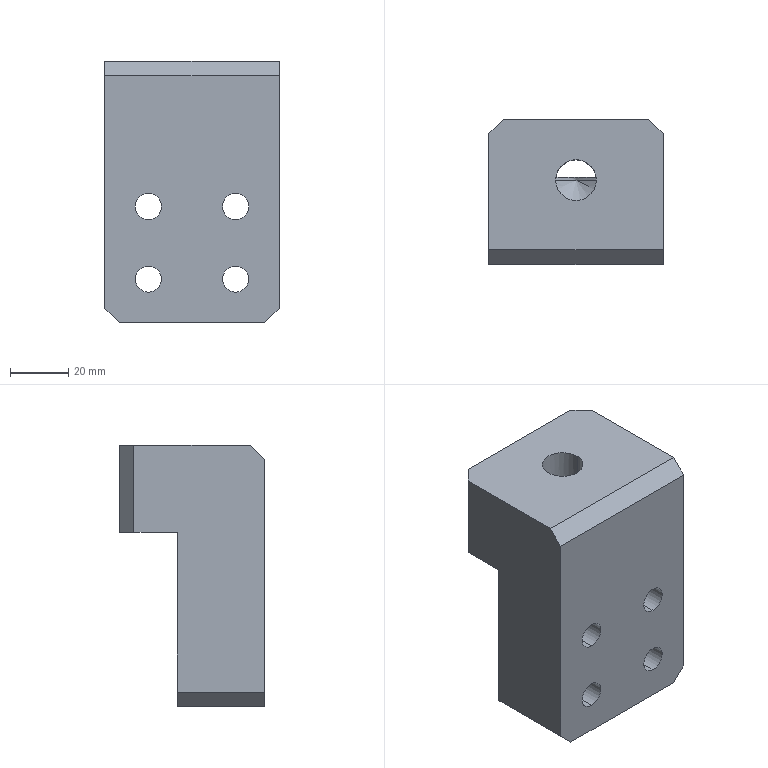Part | SolidWorks | features Chamfer 2, HoleWzd 2, Extrusion 1, ICE 1 | 1 solid | 25 faces | box 60 x 50 x 90 mm | volume 182634 mm3 | plane 13 | cylinder 10 | cone 2 | commonest cylinder face diameters 9 x8 14 x2
STEP:
#1=CARTESIAN_POINT('',(0.,14.,47.794));
#2=VERTEX_POINT('',#1);
#3=CARTESIAN_POINT('',(7.,14.,52.));
#4=VERTEX_POINT('',#3);
#5=CARTESIAN_POINT('',(7.,14.,52.));
#6=DIRECTION('',(0.8572,0.,0.515));
#7=VECTOR('',#6,1000.);
#8=LINE('',#5,#7);
#9=EDGE_CURVE('',#2,#4,#8,.T.);
#10=ORIENTED_EDGE('',*,*,#9,.F.);
#11=CARTESIAN_POINT('',(-7.,14.,52.));
#12=VERTEX_POINT('',#11);
#13=CARTESIAN_POINT('',(-7.,14.,52.));
#14=DIRECTION('',(-0.8572,0.,0.515));
#15=VECTOR('',#14,1000.);
#16=LINE('',#13,#15);
#17=EDGE_CURVE('',#2,#12,#16,.T.);
#18=ORIENTED_EDGE('',*,*,#17,.T.);
#19=CARTESIAN_POINT('',(0.,14.,52.));
#20=DIRECTION('',(0.,0.,1.));
#21=DIRECTION('',(1.,0.,0.));
#22=AXIS2_PLACEMENT_3D('',#19,#20,#21);
#23=CIRCLE('',#22,7.);
#24=EDGE_CURVE('',#12,#4,#23,.T.);
#25=ORIENTED_EDGE('',*,*,#24,.T.);
#26=EDGE_LOOP('',(#10,#18,#25));
#27=FACE_OUTER_BOUND('',#26,.T.);
#28=CARTESIAN_POINT('',(0.,14.,52.));
#29=DIRECTION('',(0.,0.,1.));
#30=DIRECTION('',(1.,0.,0.));
#31=AXIS2_PLACEMENT_3D('',#28,#29,#30);
#32=CONICAL_SURFACE('',#31,7.,1.03);
#33=ADVANCED_FACE('',(#27),#32,.F.);
#34=ORIENTED_EDGE('',*,*,#24,.F.);
#35=CARTESIAN_POINT('',(-7.,14.,90.));
#36=VERTEX_POINT('',#35);
#37=CARTESIAN_POINT('',(-7.,14.,90.));
#38=DIRECTION('',(0.,0.,1.));
#39=VECTOR('',#38,1000.);
#40=LINE('',#37,#39);
#41=EDGE_CURVE('',#12,#36,#40,.T.);
#42=ORIENTED_EDGE('',*,*,#41,.T.);
#43=CARTESIAN_POINT('',(7.,14.,90.));
#44=VERTEX_POINT('',#43);
#45=CARTESIAN_POINT('',(0.,14.,90.));
#46=DIRECTION('',(0.,0.,1.));
#47=DIRECTION('',(1.,0.,0.));
#48=AXIS2_PLACEMENT_3D('',#45,#46,#47);
#49=CIRCLE('',#48,7.);
#50=EDGE_CURVE('',#36,#44,#49,.T.);
#51=ORIENTED_EDGE('',*,*,#50,.T.);
#52=CARTESIAN_POINT('',(7.,14.,90.));
#53=DIRECTION('',(0.,0.,1.));
#54=VECTOR('',#53,1000.);
#55=LINE('',#52,#54);
#56=EDGE_CURVE('',#4,#44,#55,.T.);
#57=ORIENTED_EDGE('',*,*,#56,.F.);
#58=EDGE_LOOP('',(#34,#42,#51,#57));
#59=FACE_OUTER_BOUND('',#58,.T.);
#60=CARTESIAN_POINT('',(0.,14.,90.));
#61=DIRECTION('',(0.,0.,1.));
#62=DIRECTION('',(1.,0.,0.));
#63=AXIS2_PLACEMENT_3D('',#60,#61,#62);
#64=CYLINDRICAL_SURFACE('',#63,7.);
#65=ADVANCED_FACE('',(#59),#64,.F.);
#66=CARTESIAN_POINT('',(-15.,-15.,10.5));
#67=VERTEX_POINT('',#66);
#68=CARTESIAN_POINT('',(-15.,-15.,19.5));
#69=VERTEX_POINT('',#68);
#70=CARTESIAN_POINT('',(-15.,-15.,15.));
#71=DIRECTION('',(0.,1.,0.));
#72=DIRECTION('',(0.,0.,1.));
#73=AXIS2_PLACEMENT_3D('',#70,#71,#72);
#74=CIRCLE('',#73,4.5);
#75=EDGE_CURVE('',#67,#69,#74,.T.);
#76=ORIENTED_EDGE('',*,*,#75,.F.);
#77=CARTESIAN_POINT('',(-15.,15.,10.5));
#78=VERTEX_POINT('',#77);
#79=CARTESIAN_POINT('',(-15.,15.,10.5));
#80=DIRECTION('',(0.,1.,0.));
#81=VECTOR('',#80,1000.);
#82=LINE('',#79,#81);
#83=EDGE_CURVE('',#67,#78,#82,.T.);
#84=ORIENTED_EDGE('',*,*,#83,.T.);
#85=CARTESIAN_POINT('',(-15.,15.,19.5));
#86=VERTEX_POINT('',#85);
#87=CARTESIAN_POINT('',(-15.,15.,15.));
#88=DIRECTION('',(0.,1.,0.));
#89=DIRECTION('',(0.,0.,1.));
#90=AXIS2_PLACEMENT_3D('',#87,#88,#89);
#91=CIRCLE('',#90,4.5);
#92=EDGE_CURVE('',#78,#86,#91,.T.);
#93=ORIENTED_EDGE('',*,*,#92,.T.);
#94=CARTESIAN_POINT('',(-15.,15.,19.5));
#95=DIRECTION('',(0.,1.,0.));
#96=VECTOR('',#95,1000.);
#97=LINE('',#94,#96);
#98=EDGE_CURVE('',#69,#86,#97,.T.);
#99=ORIENTED_EDGE('',*,*,#98,.F.);
#100=EDGE_LOOP('',(#76,#84,#93,#99));
#101=FACE_OUTER_BOUND('',#100,.T.);
#102=CARTESIAN_POINT('',(-15.,15.,15.));
#103=DIRECTION('',(0.,1.,0.));
#104=DIRECTION('',(0.,0.,1.));
#105=AXIS2_PLACEMENT_3D('',#102,#103,#104);
#106=CYLINDRICAL_SURFACE('',#105,4.5);
#107=ADVANCED_FACE('',(#101),#106,.F.);
#108=CARTESIAN_POINT('',(15.,-15.,10.5));
#109=VERTEX_POINT('',#108);
#110=CARTESIAN_POINT('',(15.,-15.,19.5));
#111=VERTEX_POINT('',#110);
#112=CARTESIAN_POINT('',(15.,-15.,15.));
#113=DIRECTION('',(0.,1.,0.));
#114=DIRECTION('',(0.,0.,1.));
#115=AXIS2_PLACEMENT_3D('',#112,#113,#114);
#116=CIRCLE('',#115,4.5);
#117=EDGE_CURVE('',#109,#111,#116,.T.);
#118=ORIENTED_EDGE('',*,*,#117,.F.);
#119=CARTESIAN_POINT('',(15.,15.,10.5));
#120=VERTEX_POINT('',#119);
#121=CARTESIAN_POINT('',(15.,15.,10.5));
#122=DIRECTION('',(0.,1.,0.));
#123=VECTOR('',#122,1000.);
#124=LINE('',#121,#123);
#125=EDGE_CURVE('',#109,#120,#124,.T.);
#126=ORIENTED_EDGE('',*,*,#125,.T.);
#127=CARTESIAN_POINT('',(15.,15.,19.5));
#128=VERTEX_POINT('',#127);
#129=CARTESIAN_POINT('',(15.,15.,15.));
#130=DIRECTION('',(0.,1.,0.));
#131=DIRECTION('',(0.,0.,1.));
#132=AXIS2_PLACEMENT_3D('',#129,#130,#131);
#133=CIRCLE('',#132,4.5);
#134=EDGE_CURVE('',#120,#128,#133,.T.);
#135=ORIENTED_EDGE('',*,*,#134,.T.);
#136=CARTESIAN_POINT('',(15.,15.,19.5));
#137=DIRECTION('',(0.,1.,0.));
#138=VECTOR('',#137,1000.);
#139=LINE('',#136,#138);
#140=EDGE_CURVE('',#111,#128,#139,.T.);
#141=ORIENTED_EDGE('',*,*,#140,.F.);
#142=EDGE_LOOP('',(#118,#126,#135,#141));
#143=FACE_OUTER_BOUND('',#142,.T.);
#144=CARTESIAN_POINT('',(15.,15.,15.));
#145=DIRECTION('',(0.,1.,0.));
#146=DIRECTION('',(0.,0.,1.));
#147=AXIS2_PLACEMENT_3D('',#144,#145,#146);
#148=CYLINDRICAL_SURFACE('',#147,4.5);
#149=ADVANCED_FACE('',(#143),#148,.F.);
#150=CARTESIAN_POINT('',(-15.,-15.,35.5));
#151=VERTEX_POINT('',#150);
#152=CARTESIAN_POINT('',(-15.,-15.,44.5));
#153=VERTEX_POINT('',#152);
#154=CARTESIAN_POINT('',(-15.,-15.,40.));
#155=DIRECTION('',(0.,1.,0.));
#156=DIRECTION('',(0.,0.,1.));
#157=AXIS2_PLACEMENT_3D('',#154,#155,#156);
#158=CIRCLE('',#157,4.5);
#159=EDGE_CURVE('',#151,#153,#158,.T.);
#160=ORIENTED_EDGE('',*,*,#159,.F.);
#161=CARTESIAN_POINT('',(-15.,15.,35.5));
#162=VERTEX_POINT('',#161);
#163=CARTESIAN_POINT('',(-15.,15.,35.5));
#164=DIRECTION('',(0.,1.,0.));
#165=VECTOR('',#164,1000.);
#166=LINE('',#163,#165);
#167=EDGE_CURVE('',#151,#162,#166,.T.);
#168=ORIENTED_EDGE('',*,*,#167,.T.);
#169=CARTESIAN_POINT('',(-15.,15.,44.5));
#170=VERTEX_POINT('',#169);
#171=CARTESIAN_POINT('',(-15.,15.,40.));
#172=DIRECTION('',(0.,1.,0.));
#173=DIRECTION('',(0.,0.,1.));
#174=AXIS2_PLACEMENT_3D('',#171,#172,#173);
#175=CIRCLE('',#174,4.5);
#176=EDGE_CURVE('',#162,#170,#175,.T.);
#177=ORIENTED_EDGE('',*,*,#176,.T.);
#178=CARTESIAN_POINT('',(-15.,15.,44.5));
#179=DIRECTION('',(0.,1.,0.));
#180=VECTOR('',#179,1000.);
#181=LINE('',#178,#180);
#182=EDGE_CURVE('',#153,#170,#181,.T.);
#183=ORIENTED_EDGE('',*,*,#182,.F.);
#184=EDGE_LOOP('',(#160,#168,#177,#183));
#185=FACE_OUTER_BOUND('',#184,.T.);
#186=CARTESIAN_POINT('',(-15.,15.,40.));
#187=DIRECTION('',(0.,1.,0.));
#188=DIRECTION('',(0.,0.,1.));
#189=AXIS2_PLACEMENT_3D('',#186,#187,#188);
#190=CYLINDRICAL_SURFACE('',#189,4.5);
#191=ADVANCED_FACE('',(#185),#190,.F.);
#192=CARTESIAN_POINT('',(15.,-15.,35.5));
#193=VERTEX_POINT('',#192);
#194=CARTESIAN_POINT('',(15.,-15.,44.5));
#195=VERTEX_POINT('',#194);
#196=CARTESIAN_POINT('',(15.,-15.,40.));
#197=DIRECTION('',(0.,1.,0.));
#198=DIRECTION('',(0.,0.,1.));
#199=AXIS2_PLACEMENT_3D('',#196,#197,#198);
#200=CIRCLE('',#199,4.5);
#201=EDGE_CURVE('',#193,#195,#200,.T.);
#202=ORIENTED_EDGE('',*,*,#201,.F.);
#203=CARTESIAN_POINT('',(15.,15.,35.5));
#204=VERTEX_POINT('',#203);
#205=CARTESIAN_POINT('',(15.,15.,35.5));
#206=DIRECTION('',(0.,1.,0.));
#207=VECTOR('',#206,1000.);
#208=LINE('',#205,#207);
#209=EDGE_CURVE('',#193,#204,#208,.T.);
#210=ORIENTED_EDGE('',*,*,#209,.T.);
#211=CARTESIAN_POINT('',(15.,15.,44.5));
#212=VERTEX_POINT('',#211);
#213=CARTESIAN_POINT('',(15.,15.,40.));
#214=DIRECTION('',(0.,1.,0.));
#215=DIRECTION('',(0.,0.,1.));
#216=AXIS2_PLACEMENT_3D('',#213,#214,#215);
#217=CIRCLE('',#216,4.5);
#218=EDGE_CURVE('',#204,#212,#217,.T.);
#219=ORIENTED_EDGE('',*,*,#218,.T.);
#220=CARTESIAN_POINT('',(15.,15.,44.5));
#221=DIRECTION('',(0.,1.,0.));
#222=VECTOR('',#221,1000.);
#223=LINE('',#220,#222);
#224=EDGE_CURVE('',#195,#212,#223,.T.);
#225=ORIENTED_EDGE('',*,*,#224,.F.);
#226=EDGE_LOOP('',(#202,#210,#219,#225));
#227=FACE_OUTER_BOUND('',#226,.T.);
#228=CARTESIAN_POINT('',(15.,15.,40.));
#229=DIRECTION('',(0.,1.,0.));
#230=DIRECTION('',(0.,0.,1.));
#231=AXIS2_PLACEMENT_3D('',#228,#229,#230);
#232=CYLINDRICAL_SURFACE('',#231,4.5);
#233=ADVANCED_FACE('',(#227),#232,.F.);
#234=CARTESIAN_POINT('',(-15.,15.,15.));
#235=DIRECTION('',(0.,1.,0.));
#236=DIRECTION('',(0.,0.,1.));
#237=AXIS2_PLACEMENT_3D('',#234,#235,#236);
#238=CIRCLE('',#237,4.5);
#239=EDGE_CURVE('',#86,#78,#238,.T.);
#240=ORIENTED_EDGE('',*,*,#239,.F.);
#241=ORIENTED_EDGE('',*,*,#92,.F.);
#242=EDGE_LOOP('',(#240,#241));
#243=FACE_BOUND('',#242,.T.);
#244=CARTESIAN_POINT('',(15.,15.,15.));
#245=DIRECTION('',(0.,1.,0.));
#246=DIRECTION('',(0.,0.,1.));
#247=AXIS2_PLACEMENT_3D('',#244,#245,#246);
#248=CIRCLE('',#247,4.5);
#249=EDGE_CURVE('',#128,#120,#248,.T.);
#250=ORIENTED_EDGE('',*,*,#249,.F.);
#251=ORIENTED_EDGE('',*,*,#134,.F.);
#252=EDGE_LOOP('',(#250,#251));
#253=FACE_BOUND('',#252,.T.);
#254=CARTESIAN_POINT('',(-15.,15.,40.));
#255=DIRECTION('',(0.,1.,0.));
#256=DIRECTION('',(0.,0.,1.));
#257=AXIS2_PLACEMENT_3D('',#254,#255,#256);
#258=CIRCLE('',#257,4.5);
#259=EDGE_CURVE('',#170,#162,#258,.T.);
#260=ORIENTED_EDGE('',*,*,#259,.F.);
#261=ORIENTED_EDGE('',*,*,#176,.F.);
#262=EDGE_LOOP('',(#260,#261));
#263=FACE_BOUND('',#262,.T.);
#264=CARTESIAN_POINT('',(15.,15.,40.));
#265=DIRECTION('',(0.,1.,0.));
#266=DIRECTION('',(0.,0.,1.));
#267=AXIS2_PLACEMENT_3D('',#264,#265,#266);
#268=CIRCLE('',#267,4.5);
#269=EDGE_CURVE('',#212,#204,#268,.T.);
#270=ORIENTED_EDGE('',*,*,#269,.F.);
#271=ORIENTED_EDGE('',*,*,#218,.F.);
#272=EDGE_LOOP('',(#270,#271));
#273=FACE_BOUND('',#272,.T.);
#274=CARTESIAN_POINT('',(25.,15.,0.));
#275=VERTEX_POINT('',#274);
#276=CARTESIAN_POINT('',(-25.,15.,0.));
#277=VERTEX_POINT('',#276);
#278=CARTESIAN_POINT('',(-30.,15.,0.));
#279=DIRECTION('',(-1.,0.,0.));
#280=VECTOR('',#279,1000.);
#281=LINE('',#278,#280);
#282=EDGE_CURVE('',#275,#277,#281,.T.);
#283=ORIENTED_EDGE('',*,*,#282,.T.);
#284=CARTESIAN_POINT('',(-30.,15.,5.));
#285=VERTEX_POINT('',#284);
#286=CARTESIAN_POINT('',(-30.,15.,5.));
#287=DIRECTION('',(-0.7071,0.,0.7071));
#288=VECTOR('',#287,1000.);
#289=LINE('',#286,#288);
#290=EDGE_CURVE('',#277,#285,#289,.T.);
#291=ORIENTED_EDGE('',*,*,#290,.T.);
#292=CARTESIAN_POINT('',(-30.,15.,60.));
#293=VERTEX_POINT('',#292);
#294=CARTESIAN_POINT('',(-30.,15.,90.));
#295=DIRECTION('',(0.,0.,-1.));
#296=VECTOR('',#295,1000.);
#297=LINE('',#294,#296);
#298=EDGE_CURVE('',#293,#285,#297,.T.);
#299=ORIENTED_EDGE('',*,*,#298,.F.);
#300=CARTESIAN_POINT('',(-6.928,15.,60.));
#301=VERTEX_POINT('',#300);
#302=CARTESIAN_POINT('',(-30.,15.,60.));
#303=DIRECTION('',(-1.,0.,0.));
#304=VECTOR('',#303,1000.);
#305=LINE('',#302,#304);
#306=EDGE_CURVE('',#301,#293,#305,.T.);
#307=ORIENTED_EDGE('',*,*,#306,.F.);
#308=CARTESIAN_POINT('',(-6.928,15.,52.));
#309=VERTEX_POINT('',#308);
#310=CARTESIAN_POINT('',(-6.928,15.,90.));
#311=DIRECTION('',(0.,0.,-1.));
#312=VECTOR('',#311,1000.);
#313=LINE('',#310,#312);
#314=EDGE_CURVE('',#301,#309,#313,.T.);
#315=ORIENTED_EDGE('',*,*,#314,.T.);
#316=CARTESIAN_POINT('',(6.928,15.,52.));
#317=VERTEX_POINT('',#316);
#318=CARTESIAN_POINT('',(-6.928,15.,52.));
#319=CARTESIAN_POINT('',(-5.8,15.,51.329));
#320=CARTESIAN_POINT('',(-4.672,15.,50.659));
#321=CARTESIAN_POINT('',(-2.969,15.,49.674));
#322=CARTESIAN_POINT('',(-2.4,15.,49.347));
#323=CARTESIAN_POINT('',(-1.529,15.,48.889));
#324=CARTESIAN_POINT('',(-1.236,15.,48.74));
#325=CARTESIAN_POINT('',(-0.6298,15.,48.491));
#326=CARTESIAN_POINT('',(-0.3109,15.,48.392));
#327=CARTESIAN_POINT('',(0.1811,15.,48.397));
#328=CARTESIAN_POINT('',(0.3447,15.,48.424));
#329=CARTESIAN_POINT('',(0.6592,15.,48.509));
#330=CARTESIAN_POINT('',(0.8132,15.,48.566));
#331=CARTESIAN_POINT('',(1.267,15.,48.755));
#332=CARTESIAN_POINT('',(1.558,15.,48.903));
#333=CARTESIAN_POINT('',(2.423,15.,49.36));
#334=CARTESIAN_POINT('',(2.989,15.,49.685));
#335=CARTESIAN_POINT('',(4.684,15.,50.666));
#336=CARTESIAN_POINT('',(5.806,15.,51.333));
#337=CARTESIAN_POINT('',(6.928,15.,52.));
#338=B_SPLINE_CURVE_WITH_KNOTS('',3,(#318,#319,#320,#321,#322,#323,#324,#325,#326,#327,#328,#329,#330,#331,#332,#333,#334,#335,#336,#337),.UNSPECIFIED.,.F.,.F.,(4,2,2,2,2,2,2,2,2,4),(0.03337,0.03731,0.03928,0.04026,0.04124,0.04174,0.04223,0.04321,0.04518,0.04912),.UNSPECIFIED.);
#339=EDGE_CURVE('',#309,#317,#338,.T.);
#340=ORIENTED_EDGE('',*,*,#339,.T.);
#341=CARTESIAN_POINT('',(6.928,15.,60.));
#342=VERTEX_POINT('',#341);
#343=CARTESIAN_POINT('',(6.928,15.,90.));
#344=DIRECTION('',(0.,0.,1.));
#345=VECTOR('',#344,1000.);
#346=LINE('',#343,#345);
#347=EDGE_CURVE('',#317,#342,#346,.T.);
#348=ORIENTED_EDGE('',*,*,#347,.T.);
#349=CARTESIAN_POINT('',(30.,15.,60.));
#350=VERTEX_POINT('',#349);
#351=CARTESIAN_POINT('',(-30.,15.,60.));
#352=DIRECTION('',(-1.,0.,0.));
#353=VECTOR('',#352,1000.);
#354=LINE('',#351,#353);
#355=EDGE_CURVE('',#350,#342,#354,.T.);
#356=ORIENTED_EDGE('',*,*,#355,.F.);
#357=CARTESIAN_POINT('',(30.,15.,5.));
#358=VERTEX_POINT('',#357);
#359=CARTESIAN_POINT('',(30.,15.,90.));
#360=DIRECTION('',(0.,0.,-1.));
#361=VECTOR('',#360,1000.);
#362=LINE('',#359,#361);
#363=EDGE_CURVE('',#350,#358,#362,.T.);
#364=ORIENTED_EDGE('',*,*,#363,.T.);
#365=CARTESIAN_POINT('',(30.,15.,5.));
#366=DIRECTION('',(-0.7071,0.,-0.7071));
#367=VECTOR('',#366,1000.);
#368=LINE('',#365,#367);
#369=EDGE_CURVE('',#358,#275,#368,.T.);
#370=ORIENTED_EDGE('',*,*,#369,.T.);
#371=EDGE_LOOP('',(#283,#291,#299,#307,#315,#340,#348,#356,#364,#370));
#372=FACE_OUTER_BOUND('',#371,.T.);
#373=CARTESIAN_POINT('',(-30.,15.,90.));
#374=DIRECTION('',(0.,-1.,0.));
#375=DIRECTION('',(0.,0.,-1.));
#376=AXIS2_PLACEMENT_3D('',#373,#374,#375);
#377=PLANE('',#376);
#378=ADVANCED_FACE('',(#243,#253,#263,#273,#372),#377,.F.);
#379=CARTESIAN_POINT('',(30.,-10.,90.));
#380=VERTEX_POINT('',#379);
#381=CARTESIAN_POINT('',(30.,30.,90.));
#382=VERTEX_POINT('',#381);
#383=CARTESIAN_POINT('',(30.,15.,90.));
#384=DIRECTION('',(0.,1.,0.));
#385=VECTOR('',#384,1000.);
#386=LINE('',#383,#385);
#387=EDGE_CURVE('',#380,#382,#386,.T.);
#388=ORIENTED_EDGE('',*,*,#387,.F.);
#389=CARTESIAN_POINT('',(30.,-15.,85.));
#390=VERTEX_POINT('',#389);
#391=CARTESIAN_POINT('',(30.,-10.,90.));
#392=DIRECTION('',(0.,-0.7071,-0.7071));
#393=VECTOR('',#392,1000.);
#394=LINE('',#391,#393);
#395=EDGE_CURVE('',#380,#390,#394,.T.);
#396=ORIENTED_EDGE('',*,*,#395,.T.);
#397=CARTESIAN_POINT('',(30.,-15.,5.));
#398=VERTEX_POINT('',#397);
#399=CARTESIAN_POINT('',(30.,-15.,90.));
#400=DIRECTION('',(0.,0.,-1.));
#401=VECTOR('',#400,1000.);
#402=LINE('',#399,#401);
#403=EDGE_CURVE('',#390,#398,#402,.T.);
#404=ORIENTED_EDGE('',*,*,#403,.T.);
#405=CARTESIAN_POINT('',(30.,15.,5.));
#406=DIRECTION('',(0.,1.,0.));
#407=VECTOR('',#406,1000.);
#408=LINE('',#405,#407);
#409=EDGE_CURVE('',#398,#358,#408,.T.);
#410=ORIENTED_EDGE('',*,*,#409,.T.);
#411=ORIENTED_EDGE('',*,*,#363,.F.);
#412=CARTESIAN_POINT('',(30.,30.,60.));
#413=VERTEX_POINT('',#412);
#414=CARTESIAN_POINT('',(30.,35.,60.));
#415=DIRECTION('',(0.,-1.,0.));
#416=VECTOR('',#415,1000.);
#417=LINE('',#414,#416);
#418=EDGE_CURVE('',#413,#350,#417,.T.);
#419=ORIENTED_EDGE('',*,*,#418,.F.);
#420=CARTESIAN_POINT('',(30.,30.,90.));
#421=DIRECTION('',(0.,0.,1.));
#422=VECTOR('',#421,1000.);
#423=LINE('',#420,#422);
#424=EDGE_CURVE('',#413,#382,#423,.T.);
#425=ORIENTED_EDGE('',*,*,#424,.T.);
#426=EDGE_LOOP('',(#388,#396,#404,#410,#411,#419,#425));
#427=FACE_OUTER_BOUND('',#426,.T.);
#428=CARTESIAN_POINT('',(30.,15.,90.));
#429=DIRECTION('',(-1.,0.,0.));
#430=DIRECTION('',(0.,-1.,0.));
#431=AXIS2_PLACEMENT_3D('',#428,#429,#430);
#432=PLANE('',#431);
#433=ADVANCED_FACE('',(#427),#432,.F.);
#434=CARTESIAN_POINT('',(-30.,-15.,85.));
#435=VERTEX_POINT('',#434);
#436=CARTESIAN_POINT('',(-30.,-15.,5.));
#437=VERTEX_POINT('',#436);
#438=CARTESIAN_POINT('',(-30.,-15.,90.));
#439=DIRECTION('',(0.,0.,-1.));
#440=VECTOR('',#439,1000.);
#441=LINE('',#438,#440);
#442=EDGE_CURVE('',#435,#437,#441,.T.);
#443=ORIENTED_EDGE('',*,*,#442,.F.);
#444=CARTESIAN_POINT('',(-30.,-10.,90.));
#445=VERTEX_POINT('',#444);
#446=CARTESIAN_POINT('',(-30.,-10.,90.));
#447=DIRECTION('',(0.,0.7071,0.7071));
#448=VECTOR('',#447,1000.);
#449=LINE('',#446,#448);
#450=EDGE_CURVE('',#435,#445,#449,.T.);
#451=ORIENTED_EDGE('',*,*,#450,.T.);
#452=CARTESIAN_POINT('',(-30.,30.,90.));
#453=VERTEX_POINT('',#452);
#454=CARTESIAN_POINT('',(-30.,15.,90.));
#455=DIRECTION('',(0.,-1.,0.));
#456=VECTOR('',#455,1000.);
#457=LINE('',#454,#456);
#458=EDGE_CURVE('',#453,#445,#457,.T.);
#459=ORIENTED_EDGE('',*,*,#458,.F.);
#460=CARTESIAN_POINT('',(-30.,30.,60.));
#461=VERTEX_POINT('',#460);
#462=CARTESIAN_POINT('',(-30.,30.,90.));
#463=DIRECTION('',(0.,0.,-1.));
#464=VECTOR('',#463,1000.);
#465=LINE('',#462,#464);
#466=EDGE_CURVE('',#453,#461,#465,.T.);
#467=ORIENTED_EDGE('',*,*,#466,.T.);
#468=CARTESIAN_POINT('',(-30.,35.,60.));
#469=DIRECTION('',(0.,-1.,0.));
#470=VECTOR('',#469,1000.);
#471=LINE('',#468,#470);
#472=EDGE_CURVE('',#461,#293,#471,.T.);
#473=ORIENTED_EDGE('',*,*,#472,.T.);
#474=ORIENTED_EDGE('',*,*,#298,.T.);
#475=CARTESIAN_POINT('',(-30.,15.,5.));
#476=DIRECTION('',(0.,-1.,0.));
#477=VECTOR('',#476,1000.);
#478=LINE('',#475,#477);
#479=EDGE_CURVE('',#285,#437,#478,.T.);
#480=ORIENTED_EDGE('',*,*,#479,.T.);
#481=EDGE_LOOP('',(#443,#451,#459,#467,#473,#474,#480));
#482=FACE_OUTER_BOUND('',#481,.T.);
#483=CARTESIAN_POINT('',(-30.,15.,90.));
#484=DIRECTION('',(1.,0.,0.));
#485=DIRECTION('',(0.,1.,0.));
#486=AXIS2_PLACEMENT_3D('',#483,#484,#485);
#487=PLANE('',#486);
#488=ADVANCED_FACE('',(#482),#487,.F.);
#489=CARTESIAN_POINT('',(-15.,-15.,15.));
#490=DIRECTION('',(0.,1.,0.));
#491=DIRECTION('',(0.,0.,1.));
#492=AXIS2_PLACEMENT_3D('',#489,#490,#491);
#493=CIRCLE('',#492,4.5);
#494=EDGE_CURVE('',#69,#67,#493,.T.);
#495=ORIENTED_EDGE('',*,*,#494,.T.);
#496=ORIENTED_EDGE('',*,*,#75,.T.);
#497=EDGE_LOOP('',(#495,#496));
#498=FACE_BOUND('',#497,.T.);
#499=CARTESIAN_POINT('',(15.,-15.,15.));
#500=DIRECTION('',(0.,1.,0.));
#501=DIRECTION('',(0.,0.,1.));
#502=AXIS2_PLACEMENT_3D('',#499,#500,#501);
#503=CIRCLE('',#502,4.5);
#504=EDGE_CURVE('',#111,#109,#503,.T.);
#505=ORIENTED_EDGE('',*,*,#504,.T.);
#506=ORIENTED_EDGE('',*,*,#117,.T.);
#507=EDGE_LOOP('',(#505,#506));
#508=FACE_BOUND('',#507,.T.);
#509=CARTESIAN_POINT('',(-15.,-15.,40.));
#510=DIRECTION('',(0.,1.,0.));
#511=DIRECTION('',(0.,0.,1.));
#512=AXIS2_PLACEMENT_3D('',#509,#510,#511);
#513=CIRCLE('',#512,4.5);
#514=EDGE_CURVE('',#153,#151,#513,.T.);
#515=ORIENTED_EDGE('',*,*,#514,.T.);
#516=ORIENTED_EDGE('',*,*,#159,.T.);
#517=EDGE_LOOP('',(#515,#516));
#518=FACE_BOUND('',#517,.T.);
#519=CARTESIAN_POINT('',(15.,-15.,40.));
#520=DIRECTION('',(0.,1.,0.));
#521=DIRECTION('',(0.,0.,1.));
#522=AXIS2_PLACEMENT_3D('',#519,#520,#521);
#523=CIRCLE('',#522,4.5);
#524=EDGE_CURVE('',#195,#193,#523,.T.);
#525=ORIENTED_EDGE('',*,*,#524,.T.);
#526=ORIENTED_EDGE('',*,*,#201,.T.);
#527=EDGE_LOOP('',(#525,#526));
#528=FACE_BOUND('',#527,.T.);
#529=ORIENTED_EDGE('',*,*,#403,.F.);
#530=CARTESIAN_POINT('',(-30.,-15.,85.));
#531=DIRECTION('',(-1.,0.,0.));
#532=VECTOR('',#531,1000.);
#533=LINE('',#530,#532);
#534=EDGE_CURVE('',#390,#435,#533,.T.);
#535=ORIENTED_EDGE('',*,*,#534,.T.);
#536=ORIENTED_EDGE('',*,*,#442,.T.);
#537=CARTESIAN_POINT('',(-25.,-15.,0.));
#538=VERTEX_POINT('',#537);
#539=CARTESIAN_POINT('',(-30.,-15.,5.));
#540=DIRECTION('',(0.7071,0.,-0.7071));
#541=VECTOR('',#540,1000.);
#542=LINE('',#539,#541);
#543=EDGE_CURVE('',#437,#538,#542,.T.);
#544=ORIENTED_EDGE('',*,*,#543,.T.);
#545=CARTESIAN_POINT('',(25.,-15.,0.));
#546=VERTEX_POINT('',#545);
#547=CARTESIAN_POINT('',(-30.,-15.,0.));
#548=DIRECTION('',(1.,0.,0.));
#549=VECTOR('',#548,1000.);
#550=LINE('',#547,#549);
#551=EDGE_CURVE('',#538,#546,#550,.T.);
#552=ORIENTED_EDGE('',*,*,#551,.T.);
#553=CARTESIAN_POINT('',(30.,-15.,5.));
#554=DIRECTION('',(0.7071,0.,0.7071));
#555=VECTOR('',#554,1000.);
#556=LINE('',#553,#555);
#557=EDGE_CURVE('',#546,#398,#556,.T.);
#558=ORIENTED_EDGE('',*,*,#557,.T.);
#559=EDGE_LOOP('',(#529,#535,#536,#544,#552,#558));
#560=FACE_OUTER_BOUND('',#559,.T.);
#561=CARTESIAN_POINT('',(-30.,-15.,90.));
#562=DIRECTION('',(0.,1.,0.));
#563=DIRECTION('',(0.,0.,1.));
#564=AXIS2_PLACEMENT_3D('',#561,#562,#563);
#565=PLANE('',#564);
#566=ADVANCED_FACE('',(#498,#508,#518,#528,#560),#565,.F.);
#567=CARTESIAN_POINT('',(0.,14.,90.));
#568=DIRECTION('',(0.,0.,1.));
#569=DIRECTION('',(1.,0.,0.));
#570=AXIS2_PLACEMENT_3D('',#567,#568,#569);
#571=CIRCLE('',#570,7.);
#572=EDGE_CURVE('',#44,#36,#571,.T.);
#573=ORIENTED_EDGE('',*,*,#572,.F.);
#574=ORIENTED_EDGE('',*,*,#50,.F.);
#575=EDGE_LOOP('',(#573,#574));
#576=FACE_BOUND('',#575,.T.);
#577=ORIENTED_EDGE('',*,*,#458,.T.);
#578=CARTESIAN_POINT('',(30.,-10.,90.));
#579=DIRECTION('',(1.,0.,0.));
#580=VECTOR('',#579,1000.);
#581=LINE('',#578,#580);
#582=EDGE_CURVE('',#445,#380,#581,.T.);
#583=ORIENTED_EDGE('',*,*,#582,.T.);
#584=ORIENTED_EDGE('',*,*,#387,.T.);
#585=CARTESIAN_POINT('',(25.,35.,90.));
#586=VERTEX_POINT('',#585);
#587=CARTESIAN_POINT('',(30.,30.,90.));
#588=DIRECTION('',(-0.7071,0.7071,0.));
#589=VECTOR('',#588,1000.);
#590=LINE('',#587,#589);
#591=EDGE_CURVE('',#382,#586,#590,.T.);
#592=ORIENTED_EDGE('',*,*,#591,.T.);
#593=CARTESIAN_POINT('',(-25.,35.,90.));
#594=VERTEX_POINT('',#593);
#595=CARTESIAN_POINT('',(-30.,35.,90.));
#596=DIRECTION('',(1.,0.,0.));
#597=VECTOR('',#596,1000.);
#598=LINE('',#595,#597);
#599=EDGE_CURVE('',#594,#586,#598,.T.);
#600=ORIENTED_EDGE('',*,*,#599,.F.);
#601=CARTESIAN_POINT('',(-30.,30.,90.));
#602=DIRECTION('',(-0.7071,-0.7071,0.));
#603=VECTOR('',#602,1000.);
#604=LINE('',#601,#603);
#605=EDGE_CURVE('',#594,#453,#604,.T.);
#606=ORIENTED_EDGE('',*,*,#605,.T.);
#607=EDGE_LOOP('',(#577,#583,#584,#592,#600,#606));
#608=FACE_OUTER_BOUND('',#607,.T.);
#609=CARTESIAN_POINT('',(0.,0.,90.));
#610=DIRECTION('',(0.,0.,1.));
#611=DIRECTION('',(1.,0.,0.));
#612=AXIS2_PLACEMENT_3D('',#609,#610,#611);
#613=PLANE('',#612);
#614=ADVANCED_FACE('',(#576,#608),#613,.T.);
#615=ORIENTED_EDGE('',*,*,#551,.F.);
#616=CARTESIAN_POINT('',(-25.,0.,0.));
#617=DIRECTION('',(0.,1.,0.));
#618=VECTOR('',#617,1000.);
#619=LINE('',#616,#618);
#620=EDGE_CURVE('',#538,#277,#619,.T.);
#621=ORIENTED_EDGE('',*,*,#620,.T.);
#622=ORIENTED_EDGE('',*,*,#282,.F.);
#623=CARTESIAN_POINT('',(25.,0.,0.));
#624=DIRECTION('',(0.,-1.,0.));
#625=VECTOR('',#624,1000.);
#626=LINE('',#623,#625);
#627=EDGE_CURVE('',#275,#546,#626,.T.);
#628=ORIENTED_EDGE('',*,*,#627,.T.);
#629=EDGE_LOOP('',(#615,#621,#622,#628));
#630=FACE_OUTER_BOUND('',#629,.T.);
#631=CARTESIAN_POINT('',(0.,0.,0.));
#632=DIRECTION('',(0.,0.,1.));
#633=DIRECTION('',(1.,0.,0.));
#634=AXIS2_PLACEMENT_3D('',#631,#632,#633);
#635=PLANE('',#634);
#636=ADVANCED_FACE('',(#630),#635,.F.);
#637=ORIENTED_EDGE('',*,*,#472,.F.);
#638=CARTESIAN_POINT('',(-25.,35.,60.));
#639=VERTEX_POINT('',#638);
#640=CARTESIAN_POINT('',(-25.,35.,60.));
#641=DIRECTION('',(0.7071,0.7071,0.));
#642=VECTOR('',#641,1000.);
#643=LINE('',#640,#642);
#644=EDGE_CURVE('',#461,#639,#643,.T.);
#645=ORIENTED_EDGE('',*,*,#644,.T.);
#646=CARTESIAN_POINT('',(25.,35.,60.));
#647=VERTEX_POINT('',#646);
#648=CARTESIAN_POINT('',(-30.,35.,60.));
#649=DIRECTION('',(-1.,0.,0.));
#650=VECTOR('',#649,1000.);
#651=LINE('',#648,#650);
#652=EDGE_CURVE('',#647,#639,#651,.T.);
#653=ORIENTED_EDGE('',*,*,#652,.F.);
#654=CARTESIAN_POINT('',(25.,35.,60.));
#655=DIRECTION('',(0.7071,-0.7071,0.));
#656=VECTOR('',#655,1000.);
#657=LINE('',#654,#656);
#658=EDGE_CURVE('',#647,#413,#657,.T.);
#659=ORIENTED_EDGE('',*,*,#658,.T.);
#660=ORIENTED_EDGE('',*,*,#418,.T.);
#661=ORIENTED_EDGE('',*,*,#355,.T.);
#662=CARTESIAN_POINT('',(0.,14.,60.));
#663=DIRECTION('',(0.,0.,1.));
#664=DIRECTION('',(1.,0.,0.));
#665=AXIS2_PLACEMENT_3D('',#662,#663,#664);
#666=CIRCLE('',#665,7.);
#667=EDGE_CURVE('',#342,#301,#666,.T.);
#668=ORIENTED_EDGE('',*,*,#667,.T.);
#669=ORIENTED_EDGE('',*,*,#306,.T.);
#670=EDGE_LOOP('',(#637,#645,#653,#659,#660,#661,#668,#669));
#671=FACE_OUTER_BOUND('',#670,.T.);
#672=CARTESIAN_POINT('',(-30.,35.,60.));
#673=DIRECTION('',(0.,0.,1.));
#674=DIRECTION('',(1.,0.,0.));
#675=AXIS2_PLACEMENT_3D('',#672,#673,#674);
#676=PLANE('',#675);
#677=ADVANCED_FACE('',(#671),#676,.F.);
#678=ORIENTED_EDGE('',*,*,#652,.T.);
#679=CARTESIAN_POINT('',(-25.,35.,0.));
#680=DIRECTION('',(0.,0.,1.));
#681=VECTOR('',#680,1000.);
#682=LINE('',#679,#681);
#683=EDGE_CURVE('',#639,#594,#682,.T.);
#684=ORIENTED_EDGE('',*,*,#683,.T.);
#685=ORIENTED_EDGE('',*,*,#599,.T.);
#686=CARTESIAN_POINT('',(25.,35.,0.));
#687=DIRECTION('',(0.,0.,-1.));
#688=VECTOR('',#687,1000.);
#689=LINE('',#686,#688);
#690=EDGE_CURVE('',#586,#647,#689,.T.);
#691=ORIENTED_EDGE('',*,*,#690,.T.);
#692=EDGE_LOOP('',(#678,#684,#685,#691));
#693=FACE_OUTER_BOUND('',#692,.T.);
#694=CARTESIAN_POINT('',(0.,35.,0.));
#695=DIRECTION('',(0.,-1.,0.));
#696=DIRECTION('',(0.,0.,-1.));
#697=AXIS2_PLACEMENT_3D('',#694,#695,#696);
#698=PLANE('',#697);
#699=ADVANCED_FACE('',(#693),#698,.F.);
#700=ORIENTED_EDGE('',*,*,#209,.F.);
#701=ORIENTED_EDGE('',*,*,#524,.F.);
#702=ORIENTED_EDGE('',*,*,#224,.T.);
#703=ORIENTED_EDGE('',*,*,#269,.T.);
#704=EDGE_LOOP('',(#700,#701,#702,#703));
#705=FACE_OUTER_BOUND('',#704,.T.);
#706=CARTESIAN_POINT('',(15.,15.,40.));
#707=DIRECTION('',(0.,1.,0.));
#708=DIRECTION('',(0.,0.,1.));
#709=AXIS2_PLACEMENT_3D('',#706,#707,#708);
#710=CYLINDRICAL_SURFACE('',#709,4.5);
#711=ADVANCED_FACE('',(#705),#710,.F.);
#712=ORIENTED_EDGE('',*,*,#167,.F.);
#713=ORIENTED_EDGE('',*,*,#514,.F.);
#714=ORIENTED_EDGE('',*,*,#182,.T.);
#715=ORIENTED_EDGE('',*,*,#259,.T.);
#716=EDGE_LOOP('',(#712,#713,#714,#715));
#717=FACE_OUTER_BOUND('',#716,.T.);
#718=CARTESIAN_POINT('',(-15.,15.,40.));
#719=DIRECTION('',(0.,1.,0.));
#720=DIRECTION('',(0.,0.,1.));
#721=AXIS2_PLACEMENT_3D('',#718,#719,#720);
#722=CYLINDRICAL_SURFACE('',#721,4.5);
#723=ADVANCED_FACE('',(#717),#722,.F.);
#724=ORIENTED_EDGE('',*,*,#125,.F.);
#725=ORIENTED_EDGE('',*,*,#504,.F.);
#726=ORIENTED_EDGE('',*,*,#140,.T.);
#727=ORIENTED_EDGE('',*,*,#249,.T.);
#728=EDGE_LOOP('',(#724,#725,#726,#727));
#729=FACE_OUTER_BOUND('',#728,.T.);
#730=CARTESIAN_POINT('',(15.,15.,15.));
#731=DIRECTION('',(0.,1.,0.));
#732=DIRECTION('',(0.,0.,1.));
#733=AXIS2_PLACEMENT_3D('',#730,#731,#732);
#734=CYLINDRICAL_SURFACE('',#733,4.5);
#735=ADVANCED_FACE('',(#729),#734,.F.);
#736=ORIENTED_EDGE('',*,*,#83,.F.);
#737=ORIENTED_EDGE('',*,*,#494,.F.);
#738=ORIENTED_EDGE('',*,*,#98,.T.);
#739=ORIENTED_EDGE('',*,*,#239,.T.);
#740=EDGE_LOOP('',(#736,#737,#738,#739));
#741=FACE_OUTER_BOUND('',#740,.T.);
#742=CARTESIAN_POINT('',(-15.,15.,15.));
#743=DIRECTION('',(0.,1.,0.));
#744=DIRECTION('',(0.,0.,1.));
#745=AXIS2_PLACEMENT_3D('',#742,#743,#744);
#746=CYLINDRICAL_SURFACE('',#745,4.5);
#747=ADVANCED_FACE('',(#741),#746,.F.);
#748=ORIENTED_EDGE('',*,*,#41,.F.);
#749=CARTESIAN_POINT('',(0.,14.,52.));
#750=DIRECTION('',(0.,0.,1.));
#751=DIRECTION('',(1.,0.,0.));
#752=AXIS2_PLACEMENT_3D('',#749,#750,#751);
#753=CIRCLE('',#752,7.);
#754=EDGE_CURVE('',#309,#12,#753,.T.);
#755=ORIENTED_EDGE('',*,*,#754,.F.);
#756=ORIENTED_EDGE('',*,*,#314,.F.);
#757=ORIENTED_EDGE('',*,*,#667,.F.);
#758=ORIENTED_EDGE('',*,*,#347,.F.);
#759=CARTESIAN_POINT('',(0.,14.,52.));
#760=DIRECTION('',(0.,0.,1.));
#761=DIRECTION('',(1.,0.,0.));
#762=AXIS2_PLACEMENT_3D('',#759,#760,#761);
#763=CIRCLE('',#762,7.);
#764=EDGE_CURVE('',#4,#317,#763,.T.);
#765=ORIENTED_EDGE('',*,*,#764,.F.);
#766=ORIENTED_EDGE('',*,*,#56,.T.);
#767=ORIENTED_EDGE('',*,*,#572,.T.);
#768=EDGE_LOOP('',(#748,#755,#756,#757,#758,#765,#766,#767));
#769=FACE_OUTER_BOUND('',#768,.T.);
#770=CARTESIAN_POINT('',(0.,14.,90.));
#771=DIRECTION('',(0.,0.,1.));
#772=DIRECTION('',(1.,0.,0.));
#773=AXIS2_PLACEMENT_3D('',#770,#771,#772);
#774=CYLINDRICAL_SURFACE('',#773,7.);
#775=ADVANCED_FACE('',(#769),#774,.F.);
#776=ORIENTED_EDGE('',*,*,#17,.F.);
#777=ORIENTED_EDGE('',*,*,#9,.T.);
#778=ORIENTED_EDGE('',*,*,#764,.T.);
#779=ORIENTED_EDGE('',*,*,#339,.F.);
#780=ORIENTED_EDGE('',*,*,#754,.T.);
#781=EDGE_LOOP('',(#776,#777,#778,#779,#780));
#782=FACE_OUTER_BOUND('',#781,.T.);
#783=CARTESIAN_POINT('',(0.,14.,52.));
#784=DIRECTION('',(0.,0.,1.));
#785=DIRECTION('',(1.,0.,0.));
#786=AXIS2_PLACEMENT_3D('',#783,#784,#785);
#787=CONICAL_SURFACE('',#786,7.,1.03);
#788=ADVANCED_FACE('',(#782),#787,.F.);
#789=ORIENTED_EDGE('',*,*,#290,.F.);
#790=ORIENTED_EDGE('',*,*,#620,.F.);
#791=ORIENTED_EDGE('',*,*,#543,.F.);
#792=ORIENTED_EDGE('',*,*,#479,.F.);
#793=EDGE_LOOP('',(#789,#790,#791,#792));
#794=FACE_OUTER_BOUND('',#793,.T.);
#795=CARTESIAN_POINT('',(-30.,15.,5.));
#796=DIRECTION('',(0.7071,0.,0.7071));
#797=DIRECTION('',(0.,-1.,0.));
#798=AXIS2_PLACEMENT_3D('',#795,#796,#797);
#799=PLANE('',#798);
#800=ADVANCED_FACE('',(#794),#799,.F.);
#801=ORIENTED_EDGE('',*,*,#557,.F.);
#802=ORIENTED_EDGE('',*,*,#627,.F.);
#803=ORIENTED_EDGE('',*,*,#369,.F.);
#804=ORIENTED_EDGE('',*,*,#409,.F.);
#805=EDGE_LOOP('',(#801,#802,#803,#804));
#806=FACE_OUTER_BOUND('',#805,.T.);
#807=CARTESIAN_POINT('',(30.,15.,5.));
#808=DIRECTION('',(-0.7071,0.,0.7071));
#809=DIRECTION('',(0.,1.,0.));
#810=AXIS2_PLACEMENT_3D('',#807,#808,#809);
#811=PLANE('',#810);
#812=ADVANCED_FACE('',(#806),#811,.F.);
#813=ORIENTED_EDGE('',*,*,#644,.F.);
#814=ORIENTED_EDGE('',*,*,#466,.F.);
#815=ORIENTED_EDGE('',*,*,#605,.F.);
#816=ORIENTED_EDGE('',*,*,#683,.F.);
#817=EDGE_LOOP('',(#813,#814,#815,#816));
#818=FACE_OUTER_BOUND('',#817,.T.);
#819=CARTESIAN_POINT('',(-25.,35.,0.));
#820=DIRECTION('',(0.7071,-0.7071,0.));
#821=DIRECTION('',(0.,0.,1.));
#822=AXIS2_PLACEMENT_3D('',#819,#820,#821);
#823=PLANE('',#822);
#824=ADVANCED_FACE('',(#818),#823,.F.);
#825=ORIENTED_EDGE('',*,*,#591,.F.);
#826=ORIENTED_EDGE('',*,*,#424,.F.);
#827=ORIENTED_EDGE('',*,*,#658,.F.);
#828=ORIENTED_EDGE('',*,*,#690,.F.);
#829=EDGE_LOOP('',(#825,#826,#827,#828));
#830=FACE_OUTER_BOUND('',#829,.T.);
#831=CARTESIAN_POINT('',(25.,35.,0.));
#832=DIRECTION('',(-0.7071,-0.7071,0.));
#833=DIRECTION('',(0.,0.,-1.));
#834=AXIS2_PLACEMENT_3D('',#831,#832,#833);
#835=PLANE('',#834);
#836=ADVANCED_FACE('',(#830),#835,.F.);
#837=ORIENTED_EDGE('',*,*,#450,.F.);
#838=ORIENTED_EDGE('',*,*,#534,.F.);
#839=ORIENTED_EDGE('',*,*,#395,.F.);
#840=ORIENTED_EDGE('',*,*,#582,.F.);
#841=EDGE_LOOP('',(#837,#838,#839,#840));
#842=FACE_OUTER_BOUND('',#841,.T.);
#843=CARTESIAN_POINT('',(0.,-10.,90.));
#844=DIRECTION('',(0.,-0.7071,0.7071));
#845=DIRECTION('',(-1.,0.,0.));
#846=AXIS2_PLACEMENT_3D('',#843,#844,#845);
#847=PLANE('',#846);
#848=ADVANCED_FACE('',(#842),#847,.T.);
#849=CLOSED_SHELL('',(#33,#65,#107,#149,#191,#233,#378,#433,#488,#566,#614,#636,#677,#699,#711,#723,#735,#747,#775,#788,#800,#812,#824,#836,#848));
#850=MANIFOLD_SOLID_BREP('',#849);
#851=CARTESIAN_POINT('',(0.,0.,0.));
#852=DIRECTION('',(0.,0.,1.));
#853=DIRECTION('',(1.,0.,0.));
#854=AXIS2_PLACEMENT_3D('',#851,#852,#853);
#855=(LENGTH_UNIT()NAMED_UNIT(*)SI_UNIT(.MILLI.,.METRE.));
#856=UNCERTAINTY_MEASURE_WITH_UNIT(LENGTH_MEASURE(0.00001),#855,'','');
#857=(NAMED_UNIT(*)PLANE_ANGLE_UNIT()SI_UNIT($,.RADIAN.));
#858=(NAMED_UNIT(*)SI_UNIT($,.STERADIAN.)SOLID_ANGLE_UNIT());
#859=(GEOMETRIC_REPRESENTATION_CONTEXT(3)GLOBAL_UNCERTAINTY_ASSIGNED_CONTEXT((#856))GLOBAL_UNIT_ASSIGNED_CONTEXT((#855,#857,#858))REPRESENTATION_CONTEXT('',''));
#860=ADVANCED_BREP_SHAPE_REPRESENTATION('',(#850,#854),#859);